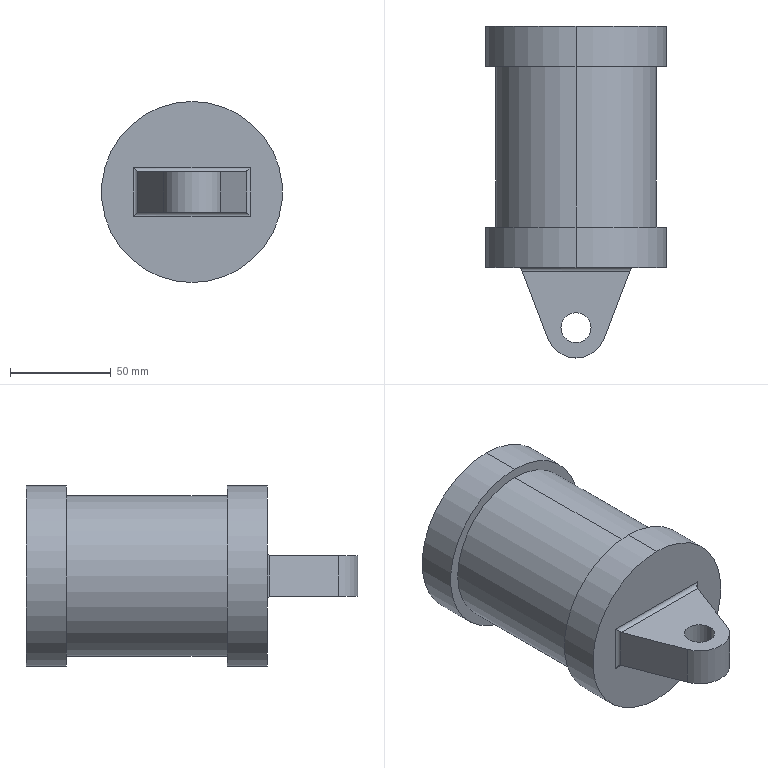Part | SolidWorks | features ICE 5, Extrusion 1, Fillet 1 | 1 solid | 27 faces | box 90 x 165 x 90 mm | volume 446114 mm3 | cylinder 17 | plane 10 | commonest cylinder face diameters 4 x4 90 x4 30 x3 15 x2 60 x2 80 x2
STEP:
#1=CARTESIAN_POINT('',(-7.5,-50.,10.));
#2=VERTEX_POINT('',#1);
#3=CARTESIAN_POINT('',(7.5,-50.,10.));
#4=VERTEX_POINT('',#3);
#5=CARTESIAN_POINT('',(0.,-50.,10.));
#6=DIRECTION('',(0.,0.,1.));
#7=DIRECTION('',(1.,0.,0.));
#8=AXIS2_PLACEMENT_3D('',#5,#6,#7);
#9=CIRCLE('',#8,7.5);
#10=EDGE_CURVE('',#2,#4,#9,.T.);
#11=ORIENTED_EDGE('',*,*,#10,.T.);
#12=CARTESIAN_POINT('',(7.5,-50.,-10.));
#13=VERTEX_POINT('',#12);
#14=CARTESIAN_POINT('',(7.5,-50.,10.));
#15=DIRECTION('',(0.,0.,-1.));
#16=VECTOR('',#15,1000.);
#17=LINE('',#14,#16);
#18=EDGE_CURVE('',#4,#13,#17,.T.);
#19=ORIENTED_EDGE('',*,*,#18,.T.);
#20=CARTESIAN_POINT('',(-7.5,-50.,-10.));
#21=VERTEX_POINT('',#20);
#22=CARTESIAN_POINT('',(0.,-50.,-10.));
#23=DIRECTION('',(0.,0.,1.));
#24=DIRECTION('',(1.,0.,0.));
#25=AXIS2_PLACEMENT_3D('',#22,#23,#24);
#26=CIRCLE('',#25,7.5);
#27=EDGE_CURVE('',#21,#13,#26,.T.);
#28=ORIENTED_EDGE('',*,*,#27,.F.);
#29=CARTESIAN_POINT('',(-7.5,-50.,10.));
#30=DIRECTION('',(0.,0.,-1.));
#31=VECTOR('',#30,1000.);
#32=LINE('',#29,#31);
#33=EDGE_CURVE('',#2,#21,#32,.T.);
#34=ORIENTED_EDGE('',*,*,#33,.F.);
#35=EDGE_LOOP('',(#11,#19,#28,#34));
#36=FACE_OUTER_BOUND('',#35,.T.);
#37=CARTESIAN_POINT('',(0.,-50.,10.));
#38=DIRECTION('',(0.,0.,-1.));
#39=DIRECTION('',(-1.,0.,0.));
#40=AXIS2_PLACEMENT_3D('',#37,#38,#39);
#41=CYLINDRICAL_SURFACE('',#40,7.5);
#42=ADVANCED_FACE('',(#36),#41,.F.);
#43=CARTESIAN_POINT('',(0.,100.,45.));
#44=VERTEX_POINT('',#43);
#45=CARTESIAN_POINT('',(0.,100.,-45.));
#46=VERTEX_POINT('',#45);
#47=CARTESIAN_POINT('',(0.,100.,0.));
#48=DIRECTION('',(0.,1.,0.));
#49=DIRECTION('',(0.,0.,1.));
#50=AXIS2_PLACEMENT_3D('',#47,#48,#49);
#51=CIRCLE('',#50,45.);
#52=EDGE_CURVE('',#44,#46,#51,.T.);
#53=ORIENTED_EDGE('',*,*,#52,.F.);
#54=CARTESIAN_POINT('',(0.,80.,45.));
#55=VERTEX_POINT('',#54);
#56=CARTESIAN_POINT('',(0.,100.,45.));
#57=DIRECTION('',(0.,-1.,0.));
#58=VECTOR('',#57,1000.);
#59=LINE('',#56,#58);
#60=EDGE_CURVE('',#44,#55,#59,.T.);
#61=ORIENTED_EDGE('',*,*,#60,.T.);
#62=CARTESIAN_POINT('',(0.,80.,-45.));
#63=VERTEX_POINT('',#62);
#64=CARTESIAN_POINT('',(0.,80.,0.));
#65=DIRECTION('',(0.,1.,0.));
#66=DIRECTION('',(0.,0.,1.));
#67=AXIS2_PLACEMENT_3D('',#64,#65,#66);
#68=CIRCLE('',#67,45.);
#69=EDGE_CURVE('',#55,#63,#68,.T.);
#70=ORIENTED_EDGE('',*,*,#69,.T.);
#71=CARTESIAN_POINT('',(0.,100.,-45.));
#72=DIRECTION('',(0.,-1.,0.));
#73=VECTOR('',#72,1000.);
#74=LINE('',#71,#73);
#75=EDGE_CURVE('',#46,#63,#74,.T.);
#76=ORIENTED_EDGE('',*,*,#75,.F.);
#77=EDGE_LOOP('',(#53,#61,#70,#76));
#78=FACE_OUTER_BOUND('',#77,.T.);
#79=CARTESIAN_POINT('',(0.,100.,0.));
#80=DIRECTION('',(0.,-1.,0.));
#81=DIRECTION('',(0.,0.,-1.));
#82=AXIS2_PLACEMENT_3D('',#79,#80,#81);
#83=CYLINDRICAL_SURFACE('',#82,45.);
#84=ADVANCED_FACE('',(#78),#83,.T.);
#85=CARTESIAN_POINT('',(0.,-20.,-45.));
#86=VERTEX_POINT('',#85);
#87=CARTESIAN_POINT('',(0.,-20.,45.));
#88=VERTEX_POINT('',#87);
#89=CARTESIAN_POINT('',(0.,-20.,0.));
#90=DIRECTION('',(0.,-1.,0.));
#91=DIRECTION('',(0.,0.,-1.));
#92=AXIS2_PLACEMENT_3D('',#89,#90,#91);
#93=CIRCLE('',#92,45.);
#94=EDGE_CURVE('',#86,#88,#93,.T.);
#95=ORIENTED_EDGE('',*,*,#94,.F.);
#96=CARTESIAN_POINT('',(0.,0.,-45.));
#97=VERTEX_POINT('',#96);
#98=CARTESIAN_POINT('',(0.,-20.,-45.));
#99=DIRECTION('',(0.,1.,0.));
#100=VECTOR('',#99,1000.);
#101=LINE('',#98,#100);
#102=EDGE_CURVE('',#86,#97,#101,.T.);
#103=ORIENTED_EDGE('',*,*,#102,.T.);
#104=CARTESIAN_POINT('',(0.,0.,45.));
#105=VERTEX_POINT('',#104);
#106=CARTESIAN_POINT('',(0.,0.,0.));
#107=DIRECTION('',(0.,-1.,0.));
#108=DIRECTION('',(0.,0.,-1.));
#109=AXIS2_PLACEMENT_3D('',#106,#107,#108);
#110=CIRCLE('',#109,45.);
#111=EDGE_CURVE('',#97,#105,#110,.T.);
#112=ORIENTED_EDGE('',*,*,#111,.T.);
#113=CARTESIAN_POINT('',(0.,-20.,45.));
#114=DIRECTION('',(0.,1.,0.));
#115=VECTOR('',#114,1000.);
#116=LINE('',#113,#115);
#117=EDGE_CURVE('',#88,#105,#116,.T.);
#118=ORIENTED_EDGE('',*,*,#117,.F.);
#119=EDGE_LOOP('',(#95,#103,#112,#118));
#120=FACE_OUTER_BOUND('',#119,.T.);
#121=CARTESIAN_POINT('',(0.,-20.,0.));
#122=DIRECTION('',(0.,1.,0.));
#123=DIRECTION('',(0.,0.,1.));
#124=AXIS2_PLACEMENT_3D('',#121,#122,#123);
#125=CYLINDRICAL_SURFACE('',#124,45.);
#126=ADVANCED_FACE('',(#120),#125,.T.);
#127=CARTESIAN_POINT('',(0.,80.,40.));
#128=VERTEX_POINT('',#127);
#129=CARTESIAN_POINT('',(0.,80.,-40.));
#130=VERTEX_POINT('',#129);
#131=CARTESIAN_POINT('',(0.,80.,0.));
#132=DIRECTION('',(0.,1.,0.));
#133=DIRECTION('',(0.,0.,1.));
#134=AXIS2_PLACEMENT_3D('',#131,#132,#133);
#135=CIRCLE('',#134,40.);
#136=EDGE_CURVE('',#128,#130,#135,.T.);
#137=ORIENTED_EDGE('',*,*,#136,.F.);
#138=CARTESIAN_POINT('',(0.,0.,40.));
#139=VERTEX_POINT('',#138);
#140=CARTESIAN_POINT('',(0.,80.,40.));
#141=DIRECTION('',(0.,-1.,0.));
#142=VECTOR('',#141,1000.);
#143=LINE('',#140,#142);
#144=EDGE_CURVE('',#128,#139,#143,.T.);
#145=ORIENTED_EDGE('',*,*,#144,.T.);
#146=CARTESIAN_POINT('',(0.,0.,-40.));
#147=VERTEX_POINT('',#146);
#148=CARTESIAN_POINT('',(0.,0.,0.));
#149=DIRECTION('',(0.,1.,0.));
#150=DIRECTION('',(0.,0.,1.));
#151=AXIS2_PLACEMENT_3D('',#148,#149,#150);
#152=CIRCLE('',#151,40.);
#153=EDGE_CURVE('',#139,#147,#152,.T.);
#154=ORIENTED_EDGE('',*,*,#153,.T.);
#155=CARTESIAN_POINT('',(0.,80.,-40.));
#156=DIRECTION('',(0.,-1.,0.));
#157=VECTOR('',#156,1000.);
#158=LINE('',#155,#157);
#159=EDGE_CURVE('',#130,#147,#158,.T.);
#160=ORIENTED_EDGE('',*,*,#159,.F.);
#161=EDGE_LOOP('',(#137,#145,#154,#160));
#162=FACE_OUTER_BOUND('',#161,.T.);
#163=CARTESIAN_POINT('',(0.,80.,0.));
#164=DIRECTION('',(0.,-1.,0.));
#165=DIRECTION('',(0.,0.,-1.));
#166=AXIS2_PLACEMENT_3D('',#163,#164,#165);
#167=CYLINDRICAL_SURFACE('',#166,40.);
#168=ADVANCED_FACE('',(#162),#167,.T.);
#169=CARTESIAN_POINT('',(0.,80.,-15.));
#170=VERTEX_POINT('',#169);
#171=CARTESIAN_POINT('',(0.,80.,15.));
#172=VERTEX_POINT('',#171);
#173=CARTESIAN_POINT('',(0.,80.,0.));
#174=DIRECTION('',(0.,1.,0.));
#175=DIRECTION('',(0.,0.,1.));
#176=AXIS2_PLACEMENT_3D('',#173,#174,#175);
#177=CIRCLE('',#176,15.);
#178=EDGE_CURVE('',#170,#172,#177,.T.);
#179=ORIENTED_EDGE('',*,*,#178,.F.);
#180=CARTESIAN_POINT('',(0.,100.,-15.));
#181=VERTEX_POINT('',#180);
#182=CARTESIAN_POINT('',(0.,60.,-15.));
#183=DIRECTION('',(0.,1.,0.));
#184=VECTOR('',#183,1000.);
#185=LINE('',#182,#184);
#186=EDGE_CURVE('',#170,#181,#185,.T.);
#187=ORIENTED_EDGE('',*,*,#186,.T.);
#188=CARTESIAN_POINT('',(0.,100.,15.));
#189=VERTEX_POINT('',#188);
#190=CARTESIAN_POINT('',(0.,100.,0.));
#191=DIRECTION('',(0.,1.,0.));
#192=DIRECTION('',(0.,0.,1.));
#193=AXIS2_PLACEMENT_3D('',#190,#191,#192);
#194=CIRCLE('',#193,15.);
#195=EDGE_CURVE('',#181,#189,#194,.T.);
#196=ORIENTED_EDGE('',*,*,#195,.T.);
#197=CARTESIAN_POINT('',(0.,60.,15.));
#198=DIRECTION('',(0.,1.,0.));
#199=VECTOR('',#198,1000.);
#200=LINE('',#197,#199);
#201=EDGE_CURVE('',#172,#189,#200,.T.);
#202=ORIENTED_EDGE('',*,*,#201,.F.);
#203=EDGE_LOOP('',(#179,#187,#196,#202));
#204=FACE_OUTER_BOUND('',#203,.T.);
#205=CARTESIAN_POINT('',(0.,60.,0.));
#206=DIRECTION('',(0.,1.,0.));
#207=DIRECTION('',(0.,0.,1.));
#208=AXIS2_PLACEMENT_3D('',#205,#206,#207);
#209=CYLINDRICAL_SURFACE('',#208,15.);
#210=ADVANCED_FACE('',(#204),#209,.F.);
#211=CARTESIAN_POINT('',(0.,0.,-30.));
#212=VERTEX_POINT('',#211);
#213=CARTESIAN_POINT('',(0.,0.,30.));
#214=VERTEX_POINT('',#213);
#215=CARTESIAN_POINT('',(0.,0.,0.));
#216=DIRECTION('',(0.,1.,0.));
#217=DIRECTION('',(0.,0.,1.));
#218=AXIS2_PLACEMENT_3D('',#215,#216,#217);
#219=CIRCLE('',#218,30.);
#220=EDGE_CURVE('',#212,#214,#219,.T.);
#221=ORIENTED_EDGE('',*,*,#220,.F.);
#222=CARTESIAN_POINT('',(0.,80.,-30.));
#223=VERTEX_POINT('',#222);
#224=CARTESIAN_POINT('',(0.,0.,-30.));
#225=DIRECTION('',(0.,1.,0.));
#226=VECTOR('',#225,1000.);
#227=LINE('',#224,#226);
#228=EDGE_CURVE('',#212,#223,#227,.T.);
#229=ORIENTED_EDGE('',*,*,#228,.T.);
#230=CARTESIAN_POINT('',(0.,80.,30.));
#231=VERTEX_POINT('',#230);
#232=CARTESIAN_POINT('',(0.,80.,0.));
#233=DIRECTION('',(0.,1.,0.));
#234=DIRECTION('',(0.,0.,1.));
#235=AXIS2_PLACEMENT_3D('',#232,#233,#234);
#236=CIRCLE('',#235,30.);
#237=EDGE_CURVE('',#223,#231,#236,.T.);
#238=ORIENTED_EDGE('',*,*,#237,.T.);
#239=CARTESIAN_POINT('',(0.,0.,30.));
#240=DIRECTION('',(0.,1.,0.));
#241=VECTOR('',#240,1000.);
#242=LINE('',#239,#241);
#243=EDGE_CURVE('',#214,#231,#242,.T.);
#244=ORIENTED_EDGE('',*,*,#243,.F.);
#245=EDGE_LOOP('',(#221,#229,#238,#244));
#246=FACE_OUTER_BOUND('',#245,.T.);
#247=CARTESIAN_POINT('',(0.,0.,0.));
#248=DIRECTION('',(0.,1.,0.));
#249=DIRECTION('',(0.,0.,1.));
#250=AXIS2_PLACEMENT_3D('',#247,#248,#249);
#251=CYLINDRICAL_SURFACE('',#250,30.);
#252=ADVANCED_FACE('',(#246),#251,.F.);
#253=CARTESIAN_POINT('',(28.878,-20.,12.));
#254=VERTEX_POINT('',#253);
#255=CARTESIAN_POINT('',(28.878,-20.,-12.));
#256=VERTEX_POINT('',#255);
#257=CARTESIAN_POINT('',(28.878,-20.,0.));
#258=DIRECTION('',(0.,0.,-1.));
#259=VECTOR('',#258,1000.);
#260=LINE('',#257,#259);
#261=EDGE_CURVE('',#254,#256,#260,.T.);
#262=ORIENTED_EDGE('',*,*,#261,.T.);
#263=CARTESIAN_POINT('',(-28.878,-20.,-12.));
#264=VERTEX_POINT('',#263);
#265=CARTESIAN_POINT('',(0.,-20.,-12.));
#266=DIRECTION('',(-1.,0.,0.));
#267=VECTOR('',#266,1000.);
#268=LINE('',#265,#267);
#269=EDGE_CURVE('',#256,#264,#268,.T.);
#270=ORIENTED_EDGE('',*,*,#269,.T.);
#271=CARTESIAN_POINT('',(-28.878,-20.,12.));
#272=VERTEX_POINT('',#271);
#273=CARTESIAN_POINT('',(-28.878,-20.,0.));
#274=DIRECTION('',(0.,0.,1.));
#275=VECTOR('',#274,1000.);
#276=LINE('',#273,#275);
#277=EDGE_CURVE('',#264,#272,#276,.T.);
#278=ORIENTED_EDGE('',*,*,#277,.T.);
#279=CARTESIAN_POINT('',(27.5,-20.,12.));
#280=DIRECTION('',(1.,0.,0.));
#281=VECTOR('',#280,1000.);
#282=LINE('',#279,#281);
#283=EDGE_CURVE('',#272,#254,#282,.T.);
#284=ORIENTED_EDGE('',*,*,#283,.T.);
#285=EDGE_LOOP('',(#262,#270,#278,#284));
#286=FACE_BOUND('',#285,.T.);
#287=CARTESIAN_POINT('',(0.,-20.,0.));
#288=DIRECTION('',(0.,-1.,0.));
#289=DIRECTION('',(0.,0.,-1.));
#290=AXIS2_PLACEMENT_3D('',#287,#288,#289);
#291=CIRCLE('',#290,45.);
#292=EDGE_CURVE('',#88,#86,#291,.T.);
#293=ORIENTED_EDGE('',*,*,#292,.T.);
#294=ORIENTED_EDGE('',*,*,#94,.T.);
#295=EDGE_LOOP('',(#293,#294));
#296=FACE_OUTER_BOUND('',#295,.T.);
#297=CARTESIAN_POINT('',(0.,-20.,0.));
#298=DIRECTION('',(0.,-1.,0.));
#299=DIRECTION('',(0.,0.,-1.));
#300=AXIS2_PLACEMENT_3D('',#297,#298,#299);
#301=PLANE('',#300);
#302=ADVANCED_FACE('',(#286,#296),#301,.T.);
#303=ORIENTED_EDGE('',*,*,#228,.F.);
#304=CARTESIAN_POINT('',(0.,0.,0.));
#305=DIRECTION('',(0.,1.,0.));
#306=DIRECTION('',(0.,0.,1.));
#307=AXIS2_PLACEMENT_3D('',#304,#305,#306);
#308=CIRCLE('',#307,30.);
#309=EDGE_CURVE('',#214,#212,#308,.T.);
#310=ORIENTED_EDGE('',*,*,#309,.F.);
#311=ORIENTED_EDGE('',*,*,#243,.T.);
#312=CARTESIAN_POINT('',(0.,80.,0.));
#313=DIRECTION('',(0.,1.,0.));
#314=DIRECTION('',(0.,0.,1.));
#315=AXIS2_PLACEMENT_3D('',#312,#313,#314);
#316=CIRCLE('',#315,30.);
#317=EDGE_CURVE('',#231,#223,#316,.T.);
#318=ORIENTED_EDGE('',*,*,#317,.T.);
#319=EDGE_LOOP('',(#303,#310,#311,#318));
#320=FACE_OUTER_BOUND('',#319,.T.);
#321=CARTESIAN_POINT('',(0.,0.,0.));
#322=DIRECTION('',(0.,1.,0.));
#323=DIRECTION('',(0.,0.,1.));
#324=AXIS2_PLACEMENT_3D('',#321,#322,#323);
#325=CYLINDRICAL_SURFACE('',#324,30.);
#326=ADVANCED_FACE('',(#320),#325,.F.);
#327=ORIENTED_EDGE('',*,*,#309,.T.);
#328=ORIENTED_EDGE('',*,*,#220,.T.);
#329=EDGE_LOOP('',(#327,#328));
#330=FACE_OUTER_BOUND('',#329,.T.);
#331=CARTESIAN_POINT('',(0.,0.,0.));
#332=DIRECTION('',(0.,1.,0.));
#333=DIRECTION('',(0.,0.,1.));
#334=AXIS2_PLACEMENT_3D('',#331,#332,#333);
#335=PLANE('',#334);
#336=ADVANCED_FACE('',(#330),#335,.T.);
#337=CARTESIAN_POINT('',(0.,80.,0.));
#338=DIRECTION('',(0.,1.,0.));
#339=DIRECTION('',(0.,0.,1.));
#340=AXIS2_PLACEMENT_3D('',#337,#338,#339);
#341=CIRCLE('',#340,15.);
#342=EDGE_CURVE('',#172,#170,#341,.T.);
#343=ORIENTED_EDGE('',*,*,#342,.T.);
#344=ORIENTED_EDGE('',*,*,#178,.T.);
#345=EDGE_LOOP('',(#343,#344));
#346=FACE_BOUND('',#345,.T.);
#347=ORIENTED_EDGE('',*,*,#317,.F.);
#348=ORIENTED_EDGE('',*,*,#237,.F.);
#349=EDGE_LOOP('',(#347,#348));
#350=FACE_OUTER_BOUND('',#349,.T.);
#351=CARTESIAN_POINT('',(0.,80.,0.));
#352=DIRECTION('',(0.,1.,0.));
#353=DIRECTION('',(0.,0.,1.));
#354=AXIS2_PLACEMENT_3D('',#351,#352,#353);
#355=PLANE('',#354);
#356=ADVANCED_FACE('',(#346,#350),#355,.F.);
#357=ORIENTED_EDGE('',*,*,#186,.F.);
#358=ORIENTED_EDGE('',*,*,#342,.F.);
#359=ORIENTED_EDGE('',*,*,#201,.T.);
#360=CARTESIAN_POINT('',(0.,100.,0.));
#361=DIRECTION('',(0.,1.,0.));
#362=DIRECTION('',(0.,0.,1.));
#363=AXIS2_PLACEMENT_3D('',#360,#361,#362);
#364=CIRCLE('',#363,15.);
#365=EDGE_CURVE('',#189,#181,#364,.T.);
#366=ORIENTED_EDGE('',*,*,#365,.T.);
#367=EDGE_LOOP('',(#357,#358,#359,#366));
#368=FACE_OUTER_BOUND('',#367,.T.);
#369=CARTESIAN_POINT('',(0.,60.,0.));
#370=DIRECTION('',(0.,1.,0.));
#371=DIRECTION('',(0.,0.,1.));
#372=AXIS2_PLACEMENT_3D('',#369,#370,#371);
#373=CYLINDRICAL_SURFACE('',#372,15.);
#374=ADVANCED_FACE('',(#368),#373,.F.);
#375=ORIENTED_EDGE('',*,*,#144,.F.);
#376=CARTESIAN_POINT('',(0.,80.,0.));
#377=DIRECTION('',(0.,1.,0.));
#378=DIRECTION('',(0.,0.,1.));
#379=AXIS2_PLACEMENT_3D('',#376,#377,#378);
#380=CIRCLE('',#379,40.);
#381=EDGE_CURVE('',#130,#128,#380,.T.);
#382=ORIENTED_EDGE('',*,*,#381,.F.);
#383=ORIENTED_EDGE('',*,*,#159,.T.);
#384=CARTESIAN_POINT('',(0.,0.,0.));
#385=DIRECTION('',(0.,1.,0.));
#386=DIRECTION('',(0.,0.,1.));
#387=AXIS2_PLACEMENT_3D('',#384,#385,#386);
#388=CIRCLE('',#387,40.);
#389=EDGE_CURVE('',#147,#139,#388,.T.);
#390=ORIENTED_EDGE('',*,*,#389,.T.);
#391=EDGE_LOOP('',(#375,#382,#383,#390));
#392=FACE_OUTER_BOUND('',#391,.T.);
#393=CARTESIAN_POINT('',(0.,80.,0.));
#394=DIRECTION('',(0.,-1.,0.));
#395=DIRECTION('',(0.,0.,-1.));
#396=AXIS2_PLACEMENT_3D('',#393,#394,#395);
#397=CYLINDRICAL_SURFACE('',#396,40.);
#398=ADVANCED_FACE('',(#392),#397,.T.);
#399=ORIENTED_EDGE('',*,*,#102,.F.);
#400=ORIENTED_EDGE('',*,*,#292,.F.);
#401=ORIENTED_EDGE('',*,*,#117,.T.);
#402=CARTESIAN_POINT('',(0.,0.,0.));
#403=DIRECTION('',(0.,-1.,0.));
#404=DIRECTION('',(0.,0.,-1.));
#405=AXIS2_PLACEMENT_3D('',#402,#403,#404);
#406=CIRCLE('',#405,45.);
#407=EDGE_CURVE('',#105,#97,#406,.T.);
#408=ORIENTED_EDGE('',*,*,#407,.T.);
#409=EDGE_LOOP('',(#399,#400,#401,#408));
#410=FACE_OUTER_BOUND('',#409,.T.);
#411=CARTESIAN_POINT('',(0.,-20.,0.));
#412=DIRECTION('',(0.,1.,0.));
#413=DIRECTION('',(0.,0.,1.));
#414=AXIS2_PLACEMENT_3D('',#411,#412,#413);
#415=CYLINDRICAL_SURFACE('',#414,45.);
#416=ADVANCED_FACE('',(#410),#415,.T.);
#417=ORIENTED_EDGE('',*,*,#389,.F.);
#418=ORIENTED_EDGE('',*,*,#153,.F.);
#419=EDGE_LOOP('',(#417,#418));
#420=FACE_BOUND('',#419,.T.);
#421=ORIENTED_EDGE('',*,*,#407,.F.);
#422=ORIENTED_EDGE('',*,*,#111,.F.);
#423=EDGE_LOOP('',(#421,#422));
#424=FACE_OUTER_BOUND('',#423,.T.);
#425=CARTESIAN_POINT('',(0.,0.,0.));
#426=DIRECTION('',(0.,-1.,0.));
#427=DIRECTION('',(0.,0.,-1.));
#428=AXIS2_PLACEMENT_3D('',#425,#426,#427);
#429=PLANE('',#428);
#430=ADVANCED_FACE('',(#420,#424),#429,.F.);
#431=ORIENTED_EDGE('',*,*,#60,.F.);
#432=CARTESIAN_POINT('',(0.,100.,0.));
#433=DIRECTION('',(0.,1.,0.));
#434=DIRECTION('',(0.,0.,1.));
#435=AXIS2_PLACEMENT_3D('',#432,#433,#434);
#436=CIRCLE('',#435,45.);
#437=EDGE_CURVE('',#46,#44,#436,.T.);
#438=ORIENTED_EDGE('',*,*,#437,.F.);
#439=ORIENTED_EDGE('',*,*,#75,.T.);
#440=CARTESIAN_POINT('',(0.,80.,0.));
#441=DIRECTION('',(0.,1.,0.));
#442=DIRECTION('',(0.,0.,1.));
#443=AXIS2_PLACEMENT_3D('',#440,#441,#442);
#444=CIRCLE('',#443,45.);
#445=EDGE_CURVE('',#63,#55,#444,.T.);
#446=ORIENTED_EDGE('',*,*,#445,.T.);
#447=EDGE_LOOP('',(#431,#438,#439,#446));
#448=FACE_OUTER_BOUND('',#447,.T.);
#449=CARTESIAN_POINT('',(0.,100.,0.));
#450=DIRECTION('',(0.,-1.,0.));
#451=DIRECTION('',(0.,0.,-1.));
#452=AXIS2_PLACEMENT_3D('',#449,#450,#451);
#453=CYLINDRICAL_SURFACE('',#452,45.);
#454=ADVANCED_FACE('',(#448),#453,.T.);
#455=ORIENTED_EDGE('',*,*,#365,.F.);
#456=ORIENTED_EDGE('',*,*,#195,.F.);
#457=EDGE_LOOP('',(#455,#456));
#458=FACE_BOUND('',#457,.T.);
#459=ORIENTED_EDGE('',*,*,#437,.T.);
#460=ORIENTED_EDGE('',*,*,#52,.T.);
#461=EDGE_LOOP('',(#459,#460));
#462=FACE_OUTER_BOUND('',#461,.T.);
#463=CARTESIAN_POINT('',(0.,100.,0.));
#464=DIRECTION('',(0.,1.,0.));
#465=DIRECTION('',(0.,0.,1.));
#466=AXIS2_PLACEMENT_3D('',#463,#464,#465);
#467=PLANE('',#466);
#468=ADVANCED_FACE('',(#458,#462),#467,.T.);
#469=ORIENTED_EDGE('',*,*,#381,.T.);
#470=ORIENTED_EDGE('',*,*,#136,.T.);
#471=EDGE_LOOP('',(#469,#470));
#472=FACE_BOUND('',#471,.T.);
#473=ORIENTED_EDGE('',*,*,#445,.F.);
#474=ORIENTED_EDGE('',*,*,#69,.F.);
#475=EDGE_LOOP('',(#473,#474));
#476=FACE_OUTER_BOUND('',#475,.T.);
#477=CARTESIAN_POINT('',(0.,80.,0.));
#478=DIRECTION('',(0.,1.,0.));
#479=DIRECTION('',(0.,0.,1.));
#480=AXIS2_PLACEMENT_3D('',#477,#478,#479);
#481=PLANE('',#480);
#482=ADVANCED_FACE('',(#472,#476),#481,.F.);
#483=CARTESIAN_POINT('',(14.015,-55.347,10.));
#484=VERTEX_POINT('',#483);
#485=CARTESIAN_POINT('',(26.737,-22.,10.));
#486=VERTEX_POINT('',#485);
#487=CARTESIAN_POINT('',(14.015,-55.347,10.));
#488=DIRECTION('',(0.3565,0.9343,0.));
#489=VECTOR('',#488,1000.);
#490=LINE('',#487,#489);
#491=EDGE_CURVE('',#484,#486,#490,.T.);
#492=ORIENTED_EDGE('',*,*,#491,.T.);
#493=CARTESIAN_POINT('',(-26.737,-22.,10.));
#494=VERTEX_POINT('',#493);
#495=CARTESIAN_POINT('',(-27.5,-22.,10.));
#496=DIRECTION('',(-1.,0.,0.));
#497=VECTOR('',#496,1000.);
#498=LINE('',#495,#497);
#499=EDGE_CURVE('',#486,#494,#498,.T.);
#500=ORIENTED_EDGE('',*,*,#499,.T.);
#501=CARTESIAN_POINT('',(-14.015,-55.347,10.));
#502=VERTEX_POINT('',#501);
#503=CARTESIAN_POINT('',(-14.015,-55.347,10.));
#504=DIRECTION('',(0.3565,-0.9343,0.));
#505=VECTOR('',#504,1000.);
#506=LINE('',#503,#505);
#507=EDGE_CURVE('',#494,#502,#506,.T.);
#508=ORIENTED_EDGE('',*,*,#507,.T.);
#509=CARTESIAN_POINT('',(0.,-50.,10.));
#510=DIRECTION('',(0.,0.,1.));
#511=DIRECTION('',(1.,0.,0.));
#512=AXIS2_PLACEMENT_3D('',#509,#510,#511);
#513=CIRCLE('',#512,15.);
#514=EDGE_CURVE('',#502,#484,#513,.T.);
#515=ORIENTED_EDGE('',*,*,#514,.T.);
#516=EDGE_LOOP('',(#492,#500,#508,#515));
#517=FACE_OUTER_BOUND('',#516,.T.);
#518=ORIENTED_EDGE('',*,*,#10,.F.);
#519=CARTESIAN_POINT('',(0.,-50.,10.));
#520=DIRECTION('',(0.,0.,1.));
#521=DIRECTION('',(1.,0.,0.));
#522=AXIS2_PLACEMENT_3D('',#519,#520,#521);
#523=CIRCLE('',#522,7.5);
#524=EDGE_CURVE('',#4,#2,#523,.T.);
#525=ORIENTED_EDGE('',*,*,#524,.F.);
#526=EDGE_LOOP('',(#518,#525));
#527=FACE_BOUND('',#526,.T.);
#528=CARTESIAN_POINT('',(0.,-50.,10.));
#529=DIRECTION('',(0.,0.,1.));
#530=DIRECTION('',(1.,0.,0.));
#531=AXIS2_PLACEMENT_3D('',#528,#529,#530);
#532=PLANE('',#531);
#533=ADVANCED_FACE('',(#517,#527),#532,.T.);
#534=CARTESIAN_POINT('',(-26.737,-22.,-10.));
#535=VERTEX_POINT('',#534);
#536=CARTESIAN_POINT('',(-14.015,-55.347,-10.));
#537=VERTEX_POINT('',#536);
#538=CARTESIAN_POINT('',(-14.015,-55.347,-10.));
#539=DIRECTION('',(0.3565,-0.9343,0.));
#540=VECTOR('',#539,1000.);
#541=LINE('',#538,#540);
#542=EDGE_CURVE('',#535,#537,#541,.T.);
#543=ORIENTED_EDGE('',*,*,#542,.F.);
#544=CARTESIAN_POINT('',(26.737,-22.,-10.));
#545=VERTEX_POINT('',#544);
#546=CARTESIAN_POINT('',(0.,-22.,-10.));
#547=DIRECTION('',(1.,0.,0.));
#548=VECTOR('',#547,1000.);
#549=LINE('',#546,#548);
#550=EDGE_CURVE('',#535,#545,#549,.T.);
#551=ORIENTED_EDGE('',*,*,#550,.T.);
#552=CARTESIAN_POINT('',(14.015,-55.347,-10.));
#553=VERTEX_POINT('',#552);
#554=CARTESIAN_POINT('',(14.015,-55.347,-10.));
#555=DIRECTION('',(0.3565,0.9343,0.));
#556=VECTOR('',#555,1000.);
#557=LINE('',#554,#556);
#558=EDGE_CURVE('',#553,#545,#557,.T.);
#559=ORIENTED_EDGE('',*,*,#558,.F.);
#560=CARTESIAN_POINT('',(0.,-50.,-10.));
#561=DIRECTION('',(0.,0.,1.));
#562=DIRECTION('',(1.,0.,0.));
#563=AXIS2_PLACEMENT_3D('',#560,#561,#562);
#564=CIRCLE('',#563,15.);
#565=EDGE_CURVE('',#537,#553,#564,.T.);
#566=ORIENTED_EDGE('',*,*,#565,.F.);
#567=EDGE_LOOP('',(#543,#551,#559,#566));
#568=FACE_OUTER_BOUND('',#567,.T.);
#569=ORIENTED_EDGE('',*,*,#27,.T.);
#570=CARTESIAN_POINT('',(0.,-50.,-10.));
#571=DIRECTION('',(0.,0.,1.));
#572=DIRECTION('',(1.,0.,0.));
#573=AXIS2_PLACEMENT_3D('',#570,#571,#572);
#574=CIRCLE('',#573,7.5);
#575=EDGE_CURVE('',#13,#21,#574,.T.);
#576=ORIENTED_EDGE('',*,*,#575,.T.);
#577=EDGE_LOOP('',(#569,#576));
#578=FACE_BOUND('',#577,.T.);
#579=CARTESIAN_POINT('',(0.,-50.,-10.));
#580=DIRECTION('',(0.,0.,1.));
#581=DIRECTION('',(1.,0.,0.));
#582=AXIS2_PLACEMENT_3D('',#579,#580,#581);
#583=PLANE('',#582);
#584=ADVANCED_FACE('',(#568,#578),#583,.F.);
#585=ORIENTED_EDGE('',*,*,#565,.T.);
#586=CARTESIAN_POINT('',(14.015,-55.347,10.));
#587=DIRECTION('',(0.,0.,-1.));
#588=VECTOR('',#587,1000.);
#589=LINE('',#586,#588);
#590=EDGE_CURVE('',#484,#553,#589,.T.);
#591=ORIENTED_EDGE('',*,*,#590,.F.);
#592=ORIENTED_EDGE('',*,*,#514,.F.);
#593=CARTESIAN_POINT('',(-14.015,-55.347,10.));
#594=DIRECTION('',(0.,0.,-1.));
#595=VECTOR('',#594,1000.);
#596=LINE('',#593,#595);
#597=EDGE_CURVE('',#502,#537,#596,.T.);
#598=ORIENTED_EDGE('',*,*,#597,.T.);
#599=EDGE_LOOP('',(#585,#591,#592,#598));
#600=FACE_OUTER_BOUND('',#599,.T.);
#601=CARTESIAN_POINT('',(0.,-50.,10.));
#602=DIRECTION('',(0.,0.,-1.));
#603=DIRECTION('',(-1.,0.,0.));
#604=AXIS2_PLACEMENT_3D('',#601,#602,#603);
#605=CYLINDRICAL_SURFACE('',#604,15.);
#606=ADVANCED_FACE('',(#600),#605,.T.);
#607=CARTESIAN_POINT('',(27.009,-21.287,-10.131));
#608=VERTEX_POINT('',#607);
#609=CARTESIAN_POINT('',(26.737,-22.,-10.));
#610=CARTESIAN_POINT('',(26.83,-21.756,-10.));
#611=CARTESIAN_POINT('',(26.922,-21.515,-10.044));
#612=CARTESIAN_POINT('',(27.009,-21.287,-10.131));
#613=(BOUNDED_CURVE()B_SPLINE_CURVE(3,(#609,#610,#611,#612),.UNSPECIFIED.,.F.,.F.)B_SPLINE_CURVE_WITH_KNOTS((4,4),(1.571,1.935),.UNSPECIFIED.)CURVE()GEOMETRIC_REPRESENTATION_ITEM()RATIONAL_B_SPLINE_CURVE((1.,0.989,0.989,1.))REPRESENTATION_ITEM(''));
#614=EDGE_CURVE('',#545,#608,#613,.T.);
#615=ORIENTED_EDGE('',*,*,#614,.T.);
#616=CARTESIAN_POINT('',(27.009,-21.287,10.131));
#617=VERTEX_POINT('',#616);
#618=CARTESIAN_POINT('',(27.009,-21.287,10.));
#619=DIRECTION('',(0.,0.,1.));
#620=VECTOR('',#619,1000.);
#621=LINE('',#618,#620);
#622=EDGE_CURVE('',#608,#617,#621,.T.);
#623=ORIENTED_EDGE('',*,*,#622,.T.);
#624=CARTESIAN_POINT('',(27.009,-21.287,10.131));
#625=CARTESIAN_POINT('',(26.922,-21.515,10.044));
#626=CARTESIAN_POINT('',(26.83,-21.756,10.));
#627=CARTESIAN_POINT('',(26.737,-22.,10.));
#628=(BOUNDED_CURVE()B_SPLINE_CURVE(3,(#624,#625,#626,#627),.UNSPECIFIED.,.F.,.F.)B_SPLINE_CURVE_WITH_KNOTS((4,4),(1.206,1.571),.UNSPECIFIED.)CURVE()GEOMETRIC_REPRESENTATION_ITEM()RATIONAL_B_SPLINE_CURVE((1.,0.989,0.989,1.))REPRESENTATION_ITEM(''));
#629=EDGE_CURVE('',#617,#486,#628,.T.);
#630=ORIENTED_EDGE('',*,*,#629,.T.);
#631=ORIENTED_EDGE('',*,*,#491,.F.);
#632=ORIENTED_EDGE('',*,*,#590,.T.);
#633=ORIENTED_EDGE('',*,*,#558,.T.);
#634=EDGE_LOOP('',(#615,#623,#630,#631,#632,#633));
#635=FACE_OUTER_BOUND('',#634,.T.);
#636=CARTESIAN_POINT('',(14.015,-55.347,10.));
#637=DIRECTION('',(-0.9343,0.3565,0.));
#638=DIRECTION('',(-0.3565,-0.9343,0.));
#639=AXIS2_PLACEMENT_3D('',#636,#637,#638);
#640=PLANE('',#639);
#641=ADVANCED_FACE('',(#635),#640,.F.);
#642=ORIENTED_EDGE('',*,*,#507,.F.);
#643=CARTESIAN_POINT('',(-27.009,-21.287,10.131));
#644=VERTEX_POINT('',#643);
#645=CARTESIAN_POINT('',(-26.737,-22.,10.));
#646=CARTESIAN_POINT('',(-26.83,-21.756,10.));
#647=CARTESIAN_POINT('',(-26.922,-21.515,10.044));
#648=CARTESIAN_POINT('',(-27.009,-21.287,10.131));
#649=(BOUNDED_CURVE()B_SPLINE_CURVE(3,(#645,#646,#647,#648),.UNSPECIFIED.,.F.,.F.)B_SPLINE_CURVE_WITH_KNOTS((4,4),(1.571,1.935),.UNSPECIFIED.)CURVE()GEOMETRIC_REPRESENTATION_ITEM()RATIONAL_B_SPLINE_CURVE((1.,0.989,0.989,1.))REPRESENTATION_ITEM(''));
#650=EDGE_CURVE('',#494,#644,#649,.T.);
#651=ORIENTED_EDGE('',*,*,#650,.T.);
#652=CARTESIAN_POINT('',(-27.009,-21.287,-10.131));
#653=VERTEX_POINT('',#652);
#654=CARTESIAN_POINT('',(-27.009,-21.287,10.));
#655=DIRECTION('',(0.,0.,-1.));
#656=VECTOR('',#655,1000.);
#657=LINE('',#654,#656);
#658=EDGE_CURVE('',#644,#653,#657,.T.);
#659=ORIENTED_EDGE('',*,*,#658,.T.);
#660=CARTESIAN_POINT('',(-27.009,-21.287,-10.131));
#661=CARTESIAN_POINT('',(-26.922,-21.515,-10.044));
#662=CARTESIAN_POINT('',(-26.83,-21.756,-10.));
#663=CARTESIAN_POINT('',(-26.737,-22.,-10.));
#664=(BOUNDED_CURVE()B_SPLINE_CURVE(3,(#660,#661,#662,#663),.UNSPECIFIED.,.F.,.F.)B_SPLINE_CURVE_WITH_KNOTS((4,4),(1.206,1.571),.UNSPECIFIED.)CURVE()GEOMETRIC_REPRESENTATION_ITEM()RATIONAL_B_SPLINE_CURVE((1.,0.989,0.989,1.))REPRESENTATION_ITEM(''));
#665=EDGE_CURVE('',#653,#535,#664,.T.);
#666=ORIENTED_EDGE('',*,*,#665,.T.);
#667=ORIENTED_EDGE('',*,*,#542,.T.);
#668=ORIENTED_EDGE('',*,*,#597,.F.);
#669=EDGE_LOOP('',(#642,#651,#659,#666,#667,#668));
#670=FACE_OUTER_BOUND('',#669,.T.);
#671=CARTESIAN_POINT('',(-14.015,-55.347,10.));
#672=DIRECTION('',(0.9343,0.3565,0.));
#673=DIRECTION('',(-0.3565,0.9343,0.));
#674=AXIS2_PLACEMENT_3D('',#671,#672,#673);
#675=PLANE('',#674);
#676=ADVANCED_FACE('',(#670),#675,.F.);
#677=ORIENTED_EDGE('',*,*,#18,.F.);
#678=ORIENTED_EDGE('',*,*,#524,.T.);
#679=ORIENTED_EDGE('',*,*,#33,.T.);
#680=ORIENTED_EDGE('',*,*,#575,.F.);
#681=EDGE_LOOP('',(#677,#678,#679,#680));
#682=FACE_OUTER_BOUND('',#681,.T.);
#683=CARTESIAN_POINT('',(0.,-50.,10.));
#684=DIRECTION('',(0.,0.,-1.));
#685=DIRECTION('',(-1.,0.,0.));
#686=AXIS2_PLACEMENT_3D('',#683,#684,#685);
#687=CYLINDRICAL_SURFACE('',#686,7.5);
#688=ADVANCED_FACE('',(#682),#687,.F.);
#689=ORIENTED_EDGE('',*,*,#499,.F.);
#690=ORIENTED_EDGE('',*,*,#629,.F.);
#691=CARTESIAN_POINT('',(28.878,-20.,12.));
#692=CARTESIAN_POINT('',(28.02,-20.,11.143));
#693=CARTESIAN_POINT('',(27.314,-20.486,10.437));
#694=CARTESIAN_POINT('',(27.009,-21.287,10.131));
#695=(BOUNDED_CURVE()B_SPLINE_CURVE(3,(#691,#692,#693,#694),.UNSPECIFIED.,.F.,.F.)B_SPLINE_CURVE_WITH_KNOTS((4,4),(1.571,2.777),.UNSPECIFIED.)CURVE()GEOMETRIC_REPRESENTATION_ITEM()RATIONAL_B_SPLINE_CURVE((1.,0.8824,0.8824,1.))REPRESENTATION_ITEM(''));
#696=EDGE_CURVE('',#254,#617,#695,.T.);
#697=ORIENTED_EDGE('',*,*,#696,.F.);
#698=ORIENTED_EDGE('',*,*,#283,.F.);
#699=CARTESIAN_POINT('',(-27.009,-21.287,10.131));
#700=CARTESIAN_POINT('',(-27.314,-20.486,10.437));
#701=CARTESIAN_POINT('',(-28.02,-20.,11.143));
#702=CARTESIAN_POINT('',(-28.878,-20.,12.));
#703=(BOUNDED_CURVE()B_SPLINE_CURVE(3,(#699,#700,#701,#702),.UNSPECIFIED.,.F.,.T.)B_SPLINE_CURVE_WITH_KNOTS((4,4),(0.3645,1.571),.UNSPECIFIED.)CURVE()GEOMETRIC_REPRESENTATION_ITEM()RATIONAL_B_SPLINE_CURVE((1.,0.8824,0.8824,1.))REPRESENTATION_ITEM(''));
#704=EDGE_CURVE('',#644,#272,#703,.T.);
#705=ORIENTED_EDGE('',*,*,#704,.F.);
#706=ORIENTED_EDGE('',*,*,#650,.F.);
#707=EDGE_LOOP('',(#689,#690,#697,#698,#705,#706));
#708=FACE_OUTER_BOUND('',#707,.T.);
#709=CARTESIAN_POINT('',(0.,-22.,12.));
#710=DIRECTION('',(1.,0.,0.));
#711=DIRECTION('',(0.,0.,-1.));
#712=AXIS2_PLACEMENT_3D('',#709,#710,#711);
#713=CYLINDRICAL_SURFACE('',#712,2.);
#714=ADVANCED_FACE('',(#708),#713,.F.);
#715=ORIENTED_EDGE('',*,*,#622,.F.);
#716=CARTESIAN_POINT('',(28.878,-20.,-12.));
#717=CARTESIAN_POINT('',(28.02,-20.,-11.143));
#718=CARTESIAN_POINT('',(27.314,-20.486,-10.437));
#719=CARTESIAN_POINT('',(27.009,-21.287,-10.131));
#720=(BOUNDED_CURVE()B_SPLINE_CURVE(3,(#716,#717,#718,#719),.UNSPECIFIED.,.F.,.F.)B_SPLINE_CURVE_WITH_KNOTS((4,4),(1.571,2.777),.UNSPECIFIED.)CURVE()GEOMETRIC_REPRESENTATION_ITEM()RATIONAL_B_SPLINE_CURVE((1.,0.8824,0.8824,1.))REPRESENTATION_ITEM(''));
#721=EDGE_CURVE('',#256,#608,#720,.T.);
#722=ORIENTED_EDGE('',*,*,#721,.F.);
#723=ORIENTED_EDGE('',*,*,#261,.F.);
#724=ORIENTED_EDGE('',*,*,#696,.T.);
#725=EDGE_LOOP('',(#715,#722,#723,#724));
#726=FACE_OUTER_BOUND('',#725,.T.);
#727=CARTESIAN_POINT('',(28.878,-22.,0.));
#728=DIRECTION('',(0.,0.,-1.));
#729=DIRECTION('',(-1.,0.,0.));
#730=AXIS2_PLACEMENT_3D('',#727,#728,#729);
#731=CYLINDRICAL_SURFACE('',#730,2.);
#732=ADVANCED_FACE('',(#726),#731,.F.);
#733=ORIENTED_EDGE('',*,*,#704,.T.);
#734=ORIENTED_EDGE('',*,*,#277,.F.);
#735=CARTESIAN_POINT('',(-27.009,-21.287,-10.131));
#736=CARTESIAN_POINT('',(-27.314,-20.486,-10.437));
#737=CARTESIAN_POINT('',(-28.02,-20.,-11.143));
#738=CARTESIAN_POINT('',(-28.878,-20.,-12.));
#739=(BOUNDED_CURVE()B_SPLINE_CURVE(3,(#735,#736,#737,#738),.UNSPECIFIED.,.F.,.T.)B_SPLINE_CURVE_WITH_KNOTS((4,4),(3.506,4.712),.UNSPECIFIED.)CURVE()GEOMETRIC_REPRESENTATION_ITEM()RATIONAL_B_SPLINE_CURVE((1.,0.8824,0.8824,1.))REPRESENTATION_ITEM(''));
#740=EDGE_CURVE('',#653,#264,#739,.T.);
#741=ORIENTED_EDGE('',*,*,#740,.F.);
#742=ORIENTED_EDGE('',*,*,#658,.F.);
#743=EDGE_LOOP('',(#733,#734,#741,#742));
#744=FACE_OUTER_BOUND('',#743,.T.);
#745=CARTESIAN_POINT('',(-28.878,-22.,10.));
#746=DIRECTION('',(0.,0.,-1.));
#747=DIRECTION('',(-1.,0.,0.));
#748=AXIS2_PLACEMENT_3D('',#745,#746,#747);
#749=CYLINDRICAL_SURFACE('',#748,2.);
#750=ADVANCED_FACE('',(#744),#749,.F.);
#751=ORIENTED_EDGE('',*,*,#614,.F.);
#752=ORIENTED_EDGE('',*,*,#550,.F.);
#753=ORIENTED_EDGE('',*,*,#665,.F.);
#754=ORIENTED_EDGE('',*,*,#740,.T.);
#755=ORIENTED_EDGE('',*,*,#269,.F.);
#756=ORIENTED_EDGE('',*,*,#721,.T.);
#757=EDGE_LOOP('',(#751,#752,#753,#754,#755,#756));
#758=FACE_OUTER_BOUND('',#757,.T.);
#759=CARTESIAN_POINT('',(0.,-22.,-12.));
#760=DIRECTION('',(-1.,0.,0.));
#761=DIRECTION('',(0.,0.,1.));
#762=AXIS2_PLACEMENT_3D('',#759,#760,#761);
#763=CYLINDRICAL_SURFACE('',#762,2.);
#764=ADVANCED_FACE('',(#758),#763,.F.);
#765=CLOSED_SHELL('',(#42,#84,#126,#168,#210,#252,#302,#326,#336,#356,#374,#398,#416,#430,#454,#468,#482,#533,#584,#606,#641,#676,#688,#714,#732,#750,#764));
#766=MANIFOLD_SOLID_BREP('',#765);
#767=CARTESIAN_POINT('',(0.,0.,0.));
#768=DIRECTION('',(0.,0.,1.));
#769=DIRECTION('',(1.,0.,0.));
#770=AXIS2_PLACEMENT_3D('',#767,#768,#769);
#771=(LENGTH_UNIT()NAMED_UNIT(*)SI_UNIT(.MILLI.,.METRE.));
#772=UNCERTAINTY_MEASURE_WITH_UNIT(LENGTH_MEASURE(0.00001),#771,'','');
#773=(NAMED_UNIT(*)PLANE_ANGLE_UNIT()SI_UNIT($,.RADIAN.));
#774=(NAMED_UNIT(*)SI_UNIT($,.STERADIAN.)SOLID_ANGLE_UNIT());
#775=(GEOMETRIC_REPRESENTATION_CONTEXT(3)GLOBAL_UNCERTAINTY_ASSIGNED_CONTEXT((#772))GLOBAL_UNIT_ASSIGNED_CONTEXT((#771,#773,#774))REPRESENTATION_CONTEXT('',''));
#776=ADVANCED_BREP_SHAPE_REPRESENTATION('',(#766,#770),#775);